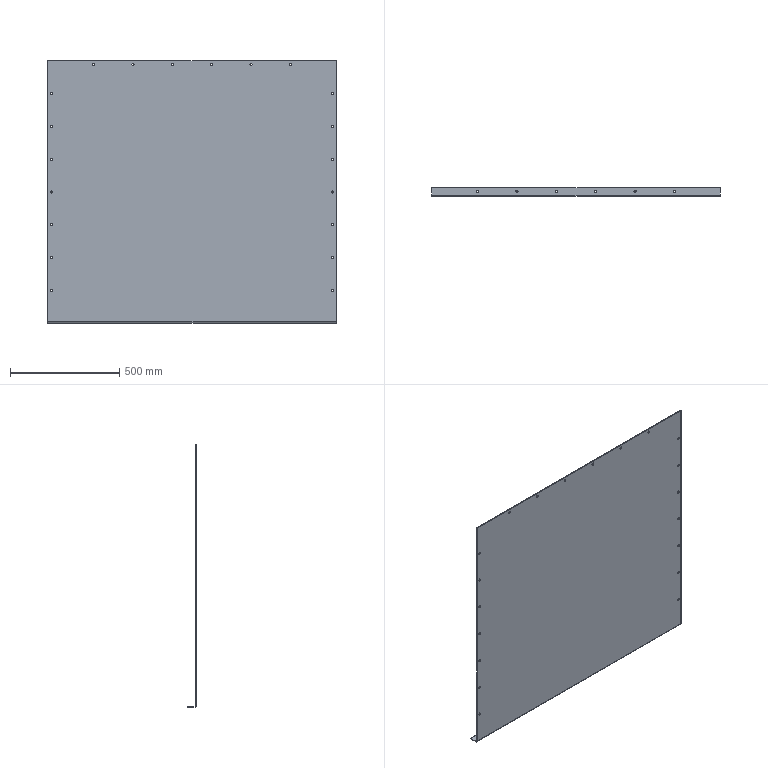Part | SolidWorks | features ICE 2, EdgeFlange 1, FlatPattern 1, SMBaseFlange 1, SheetMetal 1 | 1 solid | 66 faces | box 1320 x 40 x 1200 mm | volume 4884745 mm3 | cylinder 54 | plane 12 | commonest cylinder face diameters 10 x52 6 x1 12 x1